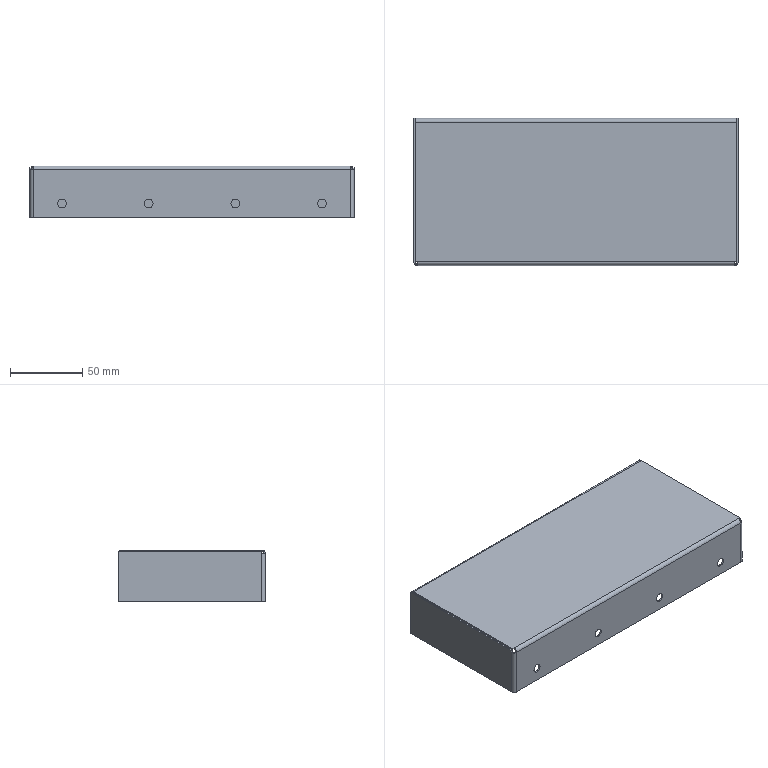Part | NX | 1 solid | 42 faces | box 225 x 102 x 36 mm | volume 44869 mm3 | plane 26 | cylinder 16 | commonest cylinder face diameters 6 x8 3.2 x4 5.2 x4
STEP:
#1=CARTESIAN_POINT('',(1610.571,113.5,87.9));
#2=VERTEX_POINT('',#1);
#3=CARTESIAN_POINT('',(1610.571,113.5,54.5));
#4=VERTEX_POINT('',#3);
#5=CARTESIAN_POINT('',(1610.571,113.5,44.938));
#6=DIRECTION('',(0.,0.,-1.));
#7=VECTOR('',#6,1000.);
#8=LINE('',#5,#7);
#9=EDGE_CURVE('',#2,#4,#8,.T.);
#10=ORIENTED_EDGE('',*,*,#9,.T.);
#11=CARTESIAN_POINT('',(1610.571,112.5,54.5));
#12=VERTEX_POINT('',#11);
#13=CARTESIAN_POINT('',(1610.571,11.5,54.5));
#14=DIRECTION('',(0.,-1.,0.));
#15=VECTOR('',#14,1000.);
#16=LINE('',#13,#15);
#17=EDGE_CURVE('',#4,#12,#16,.T.);
#18=ORIENTED_EDGE('',*,*,#17,.T.);
#19=CARTESIAN_POINT('',(1610.571,112.5,87.9));
#20=VERTEX_POINT('',#19);
#21=CARTESIAN_POINT('',(1610.571,112.5,44.938));
#22=DIRECTION('',(0.,0.,1.));
#23=VECTOR('',#22,1000.);
#24=LINE('',#21,#23);
#25=EDGE_CURVE('',#12,#20,#24,.T.);
#26=ORIENTED_EDGE('',*,*,#25,.T.);
#27=CARTESIAN_POINT('',(1610.571,110.9,89.5));
#28=VERTEX_POINT('',#27);
#29=CARTESIAN_POINT('',(1610.571,110.9,87.9));
#30=DIRECTION('',(1.,0.,0.));
#31=DIRECTION('',(0.,1.,0.));
#32=AXIS2_PLACEMENT_3D('',#29,#30,#31);
#33=CIRCLE('',#32,1.6);
#34=EDGE_CURVE('',#20,#28,#33,.T.);
#35=ORIENTED_EDGE('',*,*,#34,.T.);
#36=CARTESIAN_POINT('',(1610.571,14.1,89.5));
#37=VERTEX_POINT('',#36);
#38=CARTESIAN_POINT('',(1610.571,11.5,89.5));
#39=DIRECTION('',(0.,-1.,0.));
#40=VECTOR('',#39,1000.);
#41=LINE('',#38,#40);
#42=EDGE_CURVE('',#28,#37,#41,.T.);
#43=ORIENTED_EDGE('',*,*,#42,.T.);
#44=CARTESIAN_POINT('',(1610.571,14.1,90.5));
#45=VERTEX_POINT('',#44);
#46=CARTESIAN_POINT('',(1610.571,14.1,90.5));
#47=DIRECTION('',(0.,0.,1.));
#48=VECTOR('',#47,1000.);
#49=LINE('',#46,#48);
#50=EDGE_CURVE('',#37,#45,#49,.T.);
#51=ORIENTED_EDGE('',*,*,#50,.T.);
#52=CARTESIAN_POINT('',(1610.571,110.9,90.5));
#53=VERTEX_POINT('',#52);
#54=CARTESIAN_POINT('',(1610.571,113.5,90.5));
#55=DIRECTION('',(0.,1.,0.));
#56=VECTOR('',#55,1000.);
#57=LINE('',#54,#56);
#58=EDGE_CURVE('',#45,#53,#57,.T.);
#59=ORIENTED_EDGE('',*,*,#58,.T.);
#60=CARTESIAN_POINT('',(1610.571,110.9,87.9));
#61=DIRECTION('',(-1.,0.,0.));
#62=DIRECTION('',(0.,0.,1.));
#63=AXIS2_PLACEMENT_3D('',#60,#61,#62);
#64=CIRCLE('',#63,2.6);
#65=EDGE_CURVE('',#53,#2,#64,.T.);
#66=ORIENTED_EDGE('',*,*,#65,.T.);
#67=EDGE_LOOP('',(#10,#18,#26,#35,#43,#51,#59,#66));
#68=FACE_BOUND('',#67,.T.);
#69=CARTESIAN_POINT('',(1610.571,112.5,138.1));
#70=DIRECTION('',(-1.,0.,0.));
#71=DIRECTION('',(0.,0.,1.));
#72=AXIS2_PLACEMENT_3D('',#69,#70,#71);
#73=PLANE('',#72);
#74=ADVANCED_FACE('',(#68),#73,.T.);
#75=CARTESIAN_POINT('',(1833.5,14.1,54.5));
#76=VERTEX_POINT('',#75);
#77=CARTESIAN_POINT('',(1831.9,12.5,54.5));
#78=VERTEX_POINT('',#77);
#79=CARTESIAN_POINT('',(1831.9,14.1,54.5));
#80=DIRECTION('',(0.,0.,-1.));
#81=DIRECTION('',(1.,0.,0.));
#82=AXIS2_PLACEMENT_3D('',#79,#80,#81);
#83=CIRCLE('',#82,1.6);
#84=EDGE_CURVE('',#76,#78,#83,.T.);
#85=ORIENTED_EDGE('',*,*,#84,.F.);
#86=CARTESIAN_POINT('',(1833.5,113.5,54.5));
#87=VERTEX_POINT('',#86);
#88=CARTESIAN_POINT('',(1833.5,113.5,54.5));
#89=DIRECTION('',(0.,-1.,0.));
#90=VECTOR('',#89,1000.);
#91=LINE('',#88,#90);
#92=EDGE_CURVE('',#87,#76,#91,.T.);
#93=ORIENTED_EDGE('',*,*,#92,.F.);
#94=CARTESIAN_POINT('',(1834.5,113.5,54.5));
#95=VERTEX_POINT('',#94);
#96=CARTESIAN_POINT('',(1834.5,113.5,54.5));
#97=DIRECTION('',(-1.,0.,0.));
#98=VECTOR('',#97,1000.);
#99=LINE('',#96,#98);
#100=EDGE_CURVE('',#95,#87,#99,.T.);
#101=ORIENTED_EDGE('',*,*,#100,.F.);
#102=CARTESIAN_POINT('',(1834.5,14.1,54.5));
#103=VERTEX_POINT('',#102);
#104=CARTESIAN_POINT('',(1834.5,113.5,54.5));
#105=DIRECTION('',(0.,-1.,0.));
#106=VECTOR('',#105,1000.);
#107=LINE('',#104,#106);
#108=EDGE_CURVE('',#95,#103,#107,.T.);
#109=ORIENTED_EDGE('',*,*,#108,.T.);
#110=CARTESIAN_POINT('',(1831.9,11.5,54.5));
#111=VERTEX_POINT('',#110);
#112=CARTESIAN_POINT('',(1831.9,14.1,54.5));
#113=DIRECTION('',(0.,0.,-1.));
#114=DIRECTION('',(1.,0.,0.));
#115=AXIS2_PLACEMENT_3D('',#112,#113,#114);
#116=CIRCLE('',#115,2.6);
#117=EDGE_CURVE('',#103,#111,#116,.T.);
#118=ORIENTED_EDGE('',*,*,#117,.T.);
#119=CARTESIAN_POINT('',(1612.1,11.5,54.5));
#120=VERTEX_POINT('',#119);
#121=CARTESIAN_POINT('',(1934.4,11.5,54.5));
#122=DIRECTION('',(-1.,0.,0.));
#123=VECTOR('',#122,1000.);
#124=LINE('',#121,#123);
#125=EDGE_CURVE('',#111,#120,#124,.T.);
#126=ORIENTED_EDGE('',*,*,#125,.T.);
#127=CARTESIAN_POINT('',(1609.5,14.1,54.5));
#128=VERTEX_POINT('',#127);
#129=CARTESIAN_POINT('',(1612.1,14.1,54.5));
#130=DIRECTION('',(0.,0.,1.));
#131=DIRECTION('',(-1.,0.,0.));
#132=AXIS2_PLACEMENT_3D('',#129,#130,#131);
#133=CIRCLE('',#132,2.6);
#134=EDGE_CURVE('',#128,#120,#133,.T.);
#135=ORIENTED_EDGE('',*,*,#134,.F.);
#136=CARTESIAN_POINT('',(1609.5,113.5,54.5));
#137=VERTEX_POINT('',#136);
#138=CARTESIAN_POINT('',(1609.5,-104.365,54.5));
#139=DIRECTION('',(0.,-1.,0.));
#140=VECTOR('',#139,1000.);
#141=LINE('',#138,#140);
#142=EDGE_CURVE('',#137,#128,#141,.T.);
#143=ORIENTED_EDGE('',*,*,#142,.F.);
#144=CARTESIAN_POINT('',(1610.5,113.5,54.5));
#145=VERTEX_POINT('',#144);
#146=CARTESIAN_POINT('',(1609.5,113.5,54.5));
#147=DIRECTION('',(1.,0.,0.));
#148=VECTOR('',#147,1000.);
#149=LINE('',#146,#148);
#150=EDGE_CURVE('',#137,#145,#149,.T.);
#151=ORIENTED_EDGE('',*,*,#150,.T.);
#152=CARTESIAN_POINT('',(1610.5,14.1,54.5));
#153=VERTEX_POINT('',#152);
#154=CARTESIAN_POINT('',(1610.5,-104.365,54.5));
#155=DIRECTION('',(0.,-1.,0.));
#156=VECTOR('',#155,1000.);
#157=LINE('',#154,#156);
#158=EDGE_CURVE('',#145,#153,#157,.T.);
#159=ORIENTED_EDGE('',*,*,#158,.T.);
#160=CARTESIAN_POINT('',(1612.1,12.5,54.5));
#161=VERTEX_POINT('',#160);
#162=CARTESIAN_POINT('',(1612.1,14.1,54.5));
#163=DIRECTION('',(0.,0.,1.));
#164=DIRECTION('',(-1.,0.,0.));
#165=AXIS2_PLACEMENT_3D('',#162,#163,#164);
#166=CIRCLE('',#165,1.6);
#167=EDGE_CURVE('',#153,#161,#166,.T.);
#168=ORIENTED_EDGE('',*,*,#167,.T.);
#169=CARTESIAN_POINT('',(1934.4,12.5,54.5));
#170=DIRECTION('',(-1.,0.,0.));
#171=VECTOR('',#170,1000.);
#172=LINE('',#169,#171);
#173=EDGE_CURVE('',#78,#161,#172,.T.);
#174=ORIENTED_EDGE('',*,*,#173,.F.);
#175=EDGE_LOOP('',(#85,#93,#101,#109,#118,#126,#135,#143,#151,#159,#168,#174));
#176=FACE_BOUND('',#175,.T.);
#177=CARTESIAN_POINT('',(1831.9,14.1,54.5));
#178=DIRECTION('',(0.,0.,-1.));
#179=DIRECTION('',(0.,-1.,0.));
#180=AXIS2_PLACEMENT_3D('',#177,#178,#179);
#181=PLANE('',#180);
#182=ADVANCED_FACE('',(#176),#181,.T.);
#183=CARTESIAN_POINT('',(1833.429,112.5,54.5));
#184=VERTEX_POINT('',#183);
#185=CARTESIAN_POINT('',(1833.429,112.5,87.9));
#186=VERTEX_POINT('',#185);
#187=CARTESIAN_POINT('',(1833.429,112.5,44.938));
#188=DIRECTION('',(0.,0.,1.));
#189=VECTOR('',#188,1000.);
#190=LINE('',#187,#189);
#191=EDGE_CURVE('',#184,#186,#190,.T.);
#192=ORIENTED_EDGE('',*,*,#191,.F.);
#193=CARTESIAN_POINT('',(1833.429,113.5,54.5));
#194=VERTEX_POINT('',#193);
#195=CARTESIAN_POINT('',(1833.429,11.5,54.5));
#196=DIRECTION('',(0.,1.,0.));
#197=VECTOR('',#196,1000.);
#198=LINE('',#195,#197);
#199=EDGE_CURVE('',#184,#194,#198,.T.);
#200=ORIENTED_EDGE('',*,*,#199,.T.);
#201=CARTESIAN_POINT('',(1833.429,113.5,87.9));
#202=VERTEX_POINT('',#201);
#203=CARTESIAN_POINT('',(1833.429,113.5,44.938));
#204=DIRECTION('',(0.,0.,-1.));
#205=VECTOR('',#204,1000.);
#206=LINE('',#203,#205);
#207=EDGE_CURVE('',#202,#194,#206,.T.);
#208=ORIENTED_EDGE('',*,*,#207,.F.);
#209=CARTESIAN_POINT('',(1833.429,110.9,90.5));
#210=VERTEX_POINT('',#209);
#211=CARTESIAN_POINT('',(1833.429,110.9,87.9));
#212=DIRECTION('',(-1.,0.,0.));
#213=DIRECTION('',(0.,0.,1.));
#214=AXIS2_PLACEMENT_3D('',#211,#212,#213);
#215=CIRCLE('',#214,2.6);
#216=EDGE_CURVE('',#210,#202,#215,.T.);
#217=ORIENTED_EDGE('',*,*,#216,.F.);
#218=CARTESIAN_POINT('',(1833.429,14.1,90.5));
#219=VERTEX_POINT('',#218);
#220=CARTESIAN_POINT('',(1833.429,11.5,90.5));
#221=DIRECTION('',(0.,1.,0.));
#222=VECTOR('',#221,1000.);
#223=LINE('',#220,#222);
#224=EDGE_CURVE('',#219,#210,#223,.T.);
#225=ORIENTED_EDGE('',*,*,#224,.F.);
#226=CARTESIAN_POINT('',(1833.429,14.1,89.5));
#227=VERTEX_POINT('',#226);
#228=CARTESIAN_POINT('',(1833.429,14.1,90.5));
#229=DIRECTION('',(0.,0.,-1.));
#230=VECTOR('',#229,1000.);
#231=LINE('',#228,#230);
#232=EDGE_CURVE('',#219,#227,#231,.T.);
#233=ORIENTED_EDGE('',*,*,#232,.T.);
#234=CARTESIAN_POINT('',(1833.429,110.9,89.5));
#235=VERTEX_POINT('',#234);
#236=CARTESIAN_POINT('',(1833.429,146.329,89.5));
#237=DIRECTION('',(0.,-1.,0.));
#238=VECTOR('',#237,1000.);
#239=LINE('',#236,#238);
#240=EDGE_CURVE('',#235,#227,#239,.T.);
#241=ORIENTED_EDGE('',*,*,#240,.F.);
#242=CARTESIAN_POINT('',(1833.429,110.9,87.9));
#243=DIRECTION('',(1.,0.,0.));
#244=DIRECTION('',(0.,1.,0.));
#245=AXIS2_PLACEMENT_3D('',#242,#243,#244);
#246=CIRCLE('',#245,1.6);
#247=EDGE_CURVE('',#186,#235,#246,.T.);
#248=ORIENTED_EDGE('',*,*,#247,.F.);
#249=EDGE_LOOP('',(#192,#200,#208,#217,#225,#233,#241,#248));
#250=FACE_BOUND('',#249,.T.);
#251=CARTESIAN_POINT('',(1833.429,112.5,138.1));
#252=DIRECTION('',(1.,0.,0.));
#253=DIRECTION('',(0.,1.,0.));
#254=AXIS2_PLACEMENT_3D('',#251,#252,#253);
#255=PLANE('',#254);
#256=ADVANCED_FACE('',(#250),#255,.T.);
#257=CARTESIAN_POINT('',(1612.1,14.1,90.5));
#258=VERTEX_POINT('',#257);
#259=CARTESIAN_POINT('',(1727.465,14.1,90.5));
#260=DIRECTION('',(1.,0.,0.));
#261=VECTOR('',#260,1000.);
#262=LINE('',#259,#261);
#263=EDGE_CURVE('',#45,#258,#262,.T.);
#264=ORIENTED_EDGE('',*,*,#263,.F.);
#265=ORIENTED_EDGE('',*,*,#50,.F.);
#266=CARTESIAN_POINT('',(1612.1,14.1,89.5));
#267=VERTEX_POINT('',#266);
#268=CARTESIAN_POINT('',(1727.465,14.1,89.5));
#269=DIRECTION('',(-1.,0.,0.));
#270=VECTOR('',#269,1000.);
#271=LINE('',#268,#270);
#272=EDGE_CURVE('',#267,#37,#271,.T.);
#273=ORIENTED_EDGE('',*,*,#272,.F.);
#274=CARTESIAN_POINT('',(1612.1,14.1,90.5));
#275=DIRECTION('',(0.,0.,-1.));
#276=VECTOR('',#275,1000.);
#277=LINE('',#274,#276);
#278=EDGE_CURVE('',#258,#267,#277,.T.);
#279=ORIENTED_EDGE('',*,*,#278,.F.);
#280=EDGE_LOOP('',(#264,#265,#273,#279));
#281=FACE_BOUND('',#280,.T.);
#282=CARTESIAN_POINT('',(1609.,14.1,90.5));
#283=DIRECTION('',(0.,-1.,0.));
#284=DIRECTION('',(0.,0.,-1.));
#285=AXIS2_PLACEMENT_3D('',#282,#283,#284);
#286=PLANE('',#285);
#287=ADVANCED_FACE('',(#281),#286,.T.);
#288=CARTESIAN_POINT('',(1612.1,11.5,87.9));
#289=VERTEX_POINT('',#288);
#290=CARTESIAN_POINT('',(1609.5,14.1,87.9));
#291=VERTEX_POINT('',#290);
#292=CARTESIAN_POINT('',(1612.1,14.1,87.9));
#293=DIRECTION('',(0.,0.,-1.));
#294=DIRECTION('',(0.,-1.,0.));
#295=AXIS2_PLACEMENT_3D('',#292,#293,#294);
#296=CIRCLE('',#295,2.6);
#297=EDGE_CURVE('',#289,#291,#296,.T.);
#298=ORIENTED_EDGE('',*,*,#297,.F.);
#299=CARTESIAN_POINT('',(1612.1,12.5,87.9));
#300=VERTEX_POINT('',#299);
#301=CARTESIAN_POINT('',(1612.1,11.5,87.9));
#302=DIRECTION('',(0.,1.,0.));
#303=VECTOR('',#302,1000.);
#304=LINE('',#301,#303);
#305=EDGE_CURVE('',#289,#300,#304,.T.);
#306=ORIENTED_EDGE('',*,*,#305,.T.);
#307=CARTESIAN_POINT('',(1610.5,14.1,87.9));
#308=VERTEX_POINT('',#307);
#309=CARTESIAN_POINT('',(1612.1,14.1,87.9));
#310=DIRECTION('',(0.,0.,-1.));
#311=DIRECTION('',(0.,-1.,0.));
#312=AXIS2_PLACEMENT_3D('',#309,#310,#311);
#313=CIRCLE('',#312,1.6);
#314=EDGE_CURVE('',#300,#308,#313,.T.);
#315=ORIENTED_EDGE('',*,*,#314,.T.);
#316=CARTESIAN_POINT('',(1609.5,14.1,87.9));
#317=DIRECTION('',(1.,0.,0.));
#318=VECTOR('',#317,1000.);
#319=LINE('',#316,#318);
#320=EDGE_CURVE('',#291,#308,#319,.T.);
#321=ORIENTED_EDGE('',*,*,#320,.F.);
#322=EDGE_LOOP('',(#298,#306,#315,#321));
#323=FACE_BOUND('',#322,.T.);
#324=CARTESIAN_POINT('',(1612.1,14.1,87.9));
#325=DIRECTION('',(0.,0.,-1.));
#326=DIRECTION('',(0.,-1.,0.));
#327=AXIS2_PLACEMENT_3D('',#324,#325,#326);
#328=PLANE('',#327);
#329=ADVANCED_FACE('',(#323),#328,.F.);
#330=CARTESIAN_POINT('',(1635.,11.5,64.5));
#331=VERTEX_POINT('',#330);
#332=CARTESIAN_POINT('',(1629.,11.5,64.5));
#333=VERTEX_POINT('',#332);
#334=CARTESIAN_POINT('',(1632.,11.5,64.5));
#335=DIRECTION('',(0.,1.,0.));
#336=DIRECTION('',(1.,0.,0.));
#337=AXIS2_PLACEMENT_3D('',#334,#335,#336);
#338=CIRCLE('',#337,3.);
#339=EDGE_CURVE('',#331,#333,#338,.T.);
#340=ORIENTED_EDGE('',*,*,#339,.F.);
#341=CARTESIAN_POINT('',(1635.,12.5,64.5));
#342=VERTEX_POINT('',#341);
#343=CARTESIAN_POINT('',(1635.,12.6,64.5));
#344=DIRECTION('',(0.,1.,0.));
#345=VECTOR('',#344,1000.);
#346=LINE('',#343,#345);
#347=EDGE_CURVE('',#331,#342,#346,.T.);
#348=ORIENTED_EDGE('',*,*,#347,.T.);
#349=CARTESIAN_POINT('',(1629.,12.5,64.5));
#350=VERTEX_POINT('',#349);
#351=CARTESIAN_POINT('',(1632.,12.5,64.5));
#352=DIRECTION('',(0.,1.,0.));
#353=DIRECTION('',(1.,0.,0.));
#354=AXIS2_PLACEMENT_3D('',#351,#352,#353);
#355=CIRCLE('',#354,3.);
#356=EDGE_CURVE('',#342,#350,#355,.T.);
#357=ORIENTED_EDGE('',*,*,#356,.T.);
#358=CARTESIAN_POINT('',(1629.,12.6,64.5));
#359=DIRECTION('',(0.,1.,0.));
#360=VECTOR('',#359,1000.);
#361=LINE('',#358,#360);
#362=EDGE_CURVE('',#333,#350,#361,.T.);
#363=ORIENTED_EDGE('',*,*,#362,.F.);
#364=EDGE_LOOP('',(#340,#348,#357,#363));
#365=FACE_BOUND('',#364,.T.);
#366=CARTESIAN_POINT('',(1632.,12.6,64.5));
#367=DIRECTION('',(0.,1.,0.));
#368=DIRECTION('',(1.,0.,0.));
#369=AXIS2_PLACEMENT_3D('',#366,#367,#368);
#370=CYLINDRICAL_SURFACE('',#369,3.);
#371=ADVANCED_FACE('',(#365),#370,.F.);
#372=CARTESIAN_POINT('',(1809.,11.5,64.5));
#373=VERTEX_POINT('',#372);
#374=CARTESIAN_POINT('',(1815.,11.5,64.5));
#375=VERTEX_POINT('',#374);
#376=CARTESIAN_POINT('',(1812.,11.5,64.5));
#377=DIRECTION('',(0.,1.,0.));
#378=DIRECTION('',(1.,0.,0.));
#379=AXIS2_PLACEMENT_3D('',#376,#377,#378);
#380=CIRCLE('',#379,3.);
#381=EDGE_CURVE('',#373,#375,#380,.T.);
#382=ORIENTED_EDGE('',*,*,#381,.F.);
#383=CARTESIAN_POINT('',(1809.,12.5,64.5));
#384=VERTEX_POINT('',#383);
#385=CARTESIAN_POINT('',(1809.,12.6,64.5));
#386=DIRECTION('',(0.,1.,0.));
#387=VECTOR('',#386,1000.);
#388=LINE('',#385,#387);
#389=EDGE_CURVE('',#384,#373,#388,.F.);
#390=ORIENTED_EDGE('',*,*,#389,.F.);
#391=CARTESIAN_POINT('',(1815.,12.5,64.5));
#392=VERTEX_POINT('',#391);
#393=CARTESIAN_POINT('',(1812.,12.5,64.5));
#394=DIRECTION('',(0.,1.,0.));
#395=DIRECTION('',(1.,0.,0.));
#396=AXIS2_PLACEMENT_3D('',#393,#394,#395);
#397=CIRCLE('',#396,3.);
#398=EDGE_CURVE('',#384,#392,#397,.T.);
#399=ORIENTED_EDGE('',*,*,#398,.T.);
#400=CARTESIAN_POINT('',(1815.,12.6,64.5));
#401=DIRECTION('',(0.,1.,0.));
#402=VECTOR('',#401,1000.);
#403=LINE('',#400,#402);
#404=EDGE_CURVE('',#392,#375,#403,.F.);
#405=ORIENTED_EDGE('',*,*,#404,.T.);
#406=EDGE_LOOP('',(#382,#390,#399,#405));
#407=FACE_BOUND('',#406,.T.);
#408=CARTESIAN_POINT('',(1812.,12.6,64.5));
#409=DIRECTION('',(0.,1.,0.));
#410=DIRECTION('',(1.,0.,0.));
#411=AXIS2_PLACEMENT_3D('',#408,#409,#410);
#412=CYLINDRICAL_SURFACE('',#411,3.);
#413=ADVANCED_FACE('',(#407),#412,.F.);
#414=CARTESIAN_POINT('',(1695.,11.5,64.5));
#415=VERTEX_POINT('',#414);
#416=CARTESIAN_POINT('',(1689.,11.5,64.5));
#417=VERTEX_POINT('',#416);
#418=CARTESIAN_POINT('',(1692.,11.5,64.5));
#419=DIRECTION('',(0.,1.,0.));
#420=DIRECTION('',(1.,0.,0.));
#421=AXIS2_PLACEMENT_3D('',#418,#419,#420);
#422=CIRCLE('',#421,3.);
#423=EDGE_CURVE('',#415,#417,#422,.T.);
#424=ORIENTED_EDGE('',*,*,#423,.F.);
#425=CARTESIAN_POINT('',(1695.,12.5,64.5));
#426=VERTEX_POINT('',#425);
#427=CARTESIAN_POINT('',(1695.,12.6,64.5));
#428=DIRECTION('',(0.,1.,0.));
#429=VECTOR('',#428,1000.);
#430=LINE('',#427,#429);
#431=EDGE_CURVE('',#415,#426,#430,.T.);
#432=ORIENTED_EDGE('',*,*,#431,.T.);
#433=CARTESIAN_POINT('',(1689.,12.5,64.5));
#434=VERTEX_POINT('',#433);
#435=CARTESIAN_POINT('',(1692.,12.5,64.5));
#436=DIRECTION('',(0.,1.,0.));
#437=DIRECTION('',(1.,0.,0.));
#438=AXIS2_PLACEMENT_3D('',#435,#436,#437);
#439=CIRCLE('',#438,3.);
#440=EDGE_CURVE('',#426,#434,#439,.T.);
#441=ORIENTED_EDGE('',*,*,#440,.T.);
#442=CARTESIAN_POINT('',(1689.,12.6,64.5));
#443=DIRECTION('',(0.,1.,0.));
#444=VECTOR('',#443,1000.);
#445=LINE('',#442,#444);
#446=EDGE_CURVE('',#417,#434,#445,.T.);
#447=ORIENTED_EDGE('',*,*,#446,.F.);
#448=EDGE_LOOP('',(#424,#432,#441,#447));
#449=FACE_BOUND('',#448,.T.);
#450=CARTESIAN_POINT('',(1692.,12.6,64.5));
#451=DIRECTION('',(0.,1.,0.));
#452=DIRECTION('',(1.,0.,0.));
#453=AXIS2_PLACEMENT_3D('',#450,#451,#452);
#454=CYLINDRICAL_SURFACE('',#453,3.);
#455=ADVANCED_FACE('',(#449),#454,.F.);
#456=CARTESIAN_POINT('',(1749.,12.5,64.5));
#457=VERTEX_POINT('',#456);
#458=CARTESIAN_POINT('',(1755.,12.5,64.5));
#459=VERTEX_POINT('',#458);
#460=CARTESIAN_POINT('',(1752.,12.5,64.5));
#461=DIRECTION('',(0.,1.,0.));
#462=DIRECTION('',(1.,0.,0.));
#463=AXIS2_PLACEMENT_3D('',#460,#461,#462);
#464=CIRCLE('',#463,3.);
#465=EDGE_CURVE('',#457,#459,#464,.T.);
#466=ORIENTED_EDGE('',*,*,#465,.T.);
#467=CARTESIAN_POINT('',(1755.,11.5,64.5));
#468=VERTEX_POINT('',#467);
#469=CARTESIAN_POINT('',(1755.,12.6,64.5));
#470=DIRECTION('',(0.,1.,0.));
#471=VECTOR('',#470,1000.);
#472=LINE('',#469,#471);
#473=EDGE_CURVE('',#468,#459,#472,.T.);
#474=ORIENTED_EDGE('',*,*,#473,.F.);
#475=CARTESIAN_POINT('',(1749.,11.5,64.5));
#476=VERTEX_POINT('',#475);
#477=CARTESIAN_POINT('',(1752.,11.5,64.5));
#478=DIRECTION('',(0.,1.,0.));
#479=DIRECTION('',(1.,0.,0.));
#480=AXIS2_PLACEMENT_3D('',#477,#478,#479);
#481=CIRCLE('',#480,3.);
#482=EDGE_CURVE('',#476,#468,#481,.T.);
#483=ORIENTED_EDGE('',*,*,#482,.F.);
#484=CARTESIAN_POINT('',(1749.,12.6,64.5));
#485=DIRECTION('',(0.,1.,0.));
#486=VECTOR('',#485,1000.);
#487=LINE('',#484,#486);
#488=EDGE_CURVE('',#476,#457,#487,.T.);
#489=ORIENTED_EDGE('',*,*,#488,.T.);
#490=EDGE_LOOP('',(#466,#474,#483,#489));
#491=FACE_BOUND('',#490,.T.);
#492=CARTESIAN_POINT('',(1752.,12.6,64.5));
#493=DIRECTION('',(0.,1.,0.));
#494=DIRECTION('',(1.,0.,0.));
#495=AXIS2_PLACEMENT_3D('',#492,#493,#494);
#496=CYLINDRICAL_SURFACE('',#495,3.);
#497=ADVANCED_FACE('',(#491),#496,.F.);
#498=CARTESIAN_POINT('',(1834.5,14.1,87.9));
#499=VERTEX_POINT('',#498);
#500=CARTESIAN_POINT('',(1831.9,11.5,87.9));
#501=VERTEX_POINT('',#500);
#502=CARTESIAN_POINT('',(1831.9,14.1,87.9));
#503=DIRECTION('',(0.,0.,-1.));
#504=DIRECTION('',(1.,0.,0.));
#505=AXIS2_PLACEMENT_3D('',#502,#503,#504);
#506=CIRCLE('',#505,2.6);
#507=EDGE_CURVE('',#499,#501,#506,.T.);
#508=ORIENTED_EDGE('',*,*,#507,.F.);
#509=CARTESIAN_POINT('',(1833.5,14.1,87.9));
#510=VERTEX_POINT('',#509);
#511=CARTESIAN_POINT('',(1834.5,14.1,87.9));
#512=DIRECTION('',(-1.,0.,0.));
#513=VECTOR('',#512,1000.);
#514=LINE('',#511,#513);
#515=EDGE_CURVE('',#499,#510,#514,.T.);
#516=ORIENTED_EDGE('',*,*,#515,.T.);
#517=CARTESIAN_POINT('',(1831.9,12.5,87.9));
#518=VERTEX_POINT('',#517);
#519=CARTESIAN_POINT('',(1831.9,14.1,87.9));
#520=DIRECTION('',(0.,0.,-1.));
#521=DIRECTION('',(1.,0.,0.));
#522=AXIS2_PLACEMENT_3D('',#519,#520,#521);
#523=CIRCLE('',#522,1.6);
#524=EDGE_CURVE('',#510,#518,#523,.T.);
#525=ORIENTED_EDGE('',*,*,#524,.T.);
#526=CARTESIAN_POINT('',(1831.9,11.5,87.9));
#527=DIRECTION('',(0.,1.,0.));
#528=VECTOR('',#527,1000.);
#529=LINE('',#526,#528);
#530=EDGE_CURVE('',#501,#518,#529,.T.);
#531=ORIENTED_EDGE('',*,*,#530,.F.);
#532=EDGE_LOOP('',(#508,#516,#525,#531));
#533=FACE_BOUND('',#532,.T.);
#534=CARTESIAN_POINT('',(1831.9,14.1,87.9));
#535=DIRECTION('',(0.,0.,-1.));
#536=DIRECTION('',(0.,-1.,0.));
#537=AXIS2_PLACEMENT_3D('',#534,#535,#536);
#538=PLANE('',#537);
#539=ADVANCED_FACE('',(#533),#538,.F.);
#540=CARTESIAN_POINT('',(1831.9,14.1,90.5));
#541=VERTEX_POINT('',#540);
#542=CARTESIAN_POINT('',(1831.9,14.1,87.9));
#543=DIRECTION('',(-1.,0.,0.));
#544=DIRECTION('',(0.,-1.,0.));
#545=AXIS2_PLACEMENT_3D('',#542,#543,#544);
#546=CIRCLE('',#545,2.6);
#547=EDGE_CURVE('',#501,#541,#546,.T.);
#548=ORIENTED_EDGE('',*,*,#547,.F.);
#549=ORIENTED_EDGE('',*,*,#530,.T.);
#550=CARTESIAN_POINT('',(1831.9,14.1,89.5));
#551=VERTEX_POINT('',#550);
#552=CARTESIAN_POINT('',(1831.9,14.1,87.9));
#553=DIRECTION('',(1.,0.,0.));
#554=DIRECTION('',(0.,0.,1.));
#555=AXIS2_PLACEMENT_3D('',#552,#553,#554);
#556=CIRCLE('',#555,1.6);
#557=EDGE_CURVE('',#551,#518,#556,.T.);
#558=ORIENTED_EDGE('',*,*,#557,.F.);
#559=CARTESIAN_POINT('',(1831.9,14.1,90.5));
#560=DIRECTION('',(0.,0.,-1.));
#561=VECTOR('',#560,1000.);
#562=LINE('',#559,#561);
#563=EDGE_CURVE('',#541,#551,#562,.T.);
#564=ORIENTED_EDGE('',*,*,#563,.F.);
#565=EDGE_LOOP('',(#548,#549,#558,#564));
#566=FACE_BOUND('',#565,.T.);
#567=CARTESIAN_POINT('',(1831.9,14.1,87.9));
#568=DIRECTION('',(-1.,0.,0.));
#569=DIRECTION('',(0.,0.,1.));
#570=AXIS2_PLACEMENT_3D('',#567,#568,#569);
#571=PLANE('',#570);
#572=ADVANCED_FACE('',(#566),#571,.F.);
#573=ORIENTED_EDGE('',*,*,#547,.T.);
#574=CARTESIAN_POINT('',(1831.9,14.1,90.5));
#575=DIRECTION('',(1.,0.,0.));
#576=VECTOR('',#575,1000.);
#577=LINE('',#574,#576);
#578=EDGE_CURVE('',#258,#541,#577,.T.);
#579=ORIENTED_EDGE('',*,*,#578,.F.);
#580=CARTESIAN_POINT('',(1612.1,14.1,87.9));
#581=DIRECTION('',(1.,0.,0.));
#582=DIRECTION('',(0.,0.,1.));
#583=AXIS2_PLACEMENT_3D('',#580,#581,#582);
#584=CIRCLE('',#583,2.6);
#585=EDGE_CURVE('',#258,#289,#584,.T.);
#586=ORIENTED_EDGE('',*,*,#585,.T.);
#587=CARTESIAN_POINT('',(1727.465,11.5,87.9));
#588=DIRECTION('',(1.,0.,0.));
#589=VECTOR('',#588,1000.);
#590=LINE('',#587,#589);
#591=EDGE_CURVE('',#289,#501,#590,.T.);
#592=ORIENTED_EDGE('',*,*,#591,.T.);
#593=EDGE_LOOP('',(#573,#579,#586,#592));
#594=FACE_BOUND('',#593,.T.);
#595=CARTESIAN_POINT('',(1831.9,14.1,87.9));
#596=DIRECTION('',(1.,0.,0.));
#597=DIRECTION('',(0.,0.,-1.));
#598=AXIS2_PLACEMENT_3D('',#595,#596,#597);
#599=CYLINDRICAL_SURFACE('',#598,2.6);
#600=ADVANCED_FACE('',(#594),#599,.T.);
#601=ORIENTED_EDGE('',*,*,#207,.T.);
#602=CARTESIAN_POINT('',(1727.465,113.5,54.5));
#603=DIRECTION('',(-1.,0.,0.));
#604=VECTOR('',#603,1000.);
#605=LINE('',#602,#604);
#606=EDGE_CURVE('',#194,#4,#605,.T.);
#607=ORIENTED_EDGE('',*,*,#606,.T.);
#608=ORIENTED_EDGE('',*,*,#9,.F.);
#609=CARTESIAN_POINT('',(1727.465,113.5,87.9));
#610=DIRECTION('',(1.,0.,0.));
#611=VECTOR('',#610,1000.);
#612=LINE('',#609,#611);
#613=EDGE_CURVE('',#2,#202,#612,.T.);
#614=ORIENTED_EDGE('',*,*,#613,.T.);
#615=EDGE_LOOP('',(#601,#607,#608,#614));
#616=FACE_BOUND('',#615,.T.);
#617=CARTESIAN_POINT('',(1727.465,113.5,233.862));
#618=DIRECTION('',(0.,1.,0.));
#619=DIRECTION('',(1.,0.,0.));
#620=AXIS2_PLACEMENT_3D('',#617,#618,#619);
#621=PLANE('',#620);
#622=ADVANCED_FACE('',(#616),#621,.T.);
#623=CARTESIAN_POINT('',(1833.429,110.9,90.5));
#624=DIRECTION('',(1.,0.,0.));
#625=VECTOR('',#624,1000.);
#626=LINE('',#623,#625);
#627=EDGE_CURVE('',#53,#210,#626,.T.);
#628=ORIENTED_EDGE('',*,*,#627,.F.);
#629=ORIENTED_EDGE('',*,*,#58,.F.);
#630=ORIENTED_EDGE('',*,*,#263,.T.);
#631=ORIENTED_EDGE('',*,*,#578,.T.);
#632=CARTESIAN_POINT('',(1727.465,14.1,90.5));
#633=DIRECTION('',(1.,0.,0.));
#634=VECTOR('',#633,1000.);
#635=LINE('',#632,#634);
#636=EDGE_CURVE('',#541,#219,#635,.T.);
#637=ORIENTED_EDGE('',*,*,#636,.T.);
#638=ORIENTED_EDGE('',*,*,#224,.T.);
#639=EDGE_LOOP('',(#628,#629,#630,#631,#637,#638));
#640=FACE_BOUND('',#639,.T.);
#641=CARTESIAN_POINT('',(1727.465,-31.962,90.5));
#642=DIRECTION('',(0.,0.,1.));
#643=DIRECTION('',(1.,0.,0.));
#644=AXIS2_PLACEMENT_3D('',#641,#642,#643);
#645=PLANE('',#644);
#646=ADVANCED_FACE('',(#640),#645,.T.);
#647=ORIENTED_EDGE('',*,*,#613,.F.);
#648=ORIENTED_EDGE('',*,*,#65,.F.);
#649=ORIENTED_EDGE('',*,*,#627,.T.);
#650=ORIENTED_EDGE('',*,*,#216,.T.);
#651=EDGE_LOOP('',(#647,#648,#649,#650));
#652=FACE_BOUND('',#651,.T.);
#653=CARTESIAN_POINT('',(1833.429,110.9,87.9));
#654=DIRECTION('',(1.,0.,0.));
#655=DIRECTION('',(0.,0.,-1.));
#656=AXIS2_PLACEMENT_3D('',#653,#654,#655);
#657=CYLINDRICAL_SURFACE('',#656,2.6);
#658=ADVANCED_FACE('',(#652),#657,.T.);
#659=CARTESIAN_POINT('',(1610.5,14.1,87.9));
#660=DIRECTION('',(0.,0.,1.));
#661=VECTOR('',#660,1000.);
#662=LINE('',#659,#661);
#663=EDGE_CURVE('',#153,#308,#662,.T.);
#664=ORIENTED_EDGE('',*,*,#663,.F.);
#665=ORIENTED_EDGE('',*,*,#158,.F.);
#666=CARTESIAN_POINT('',(1610.5,113.5,89.429));
#667=VERTEX_POINT('',#666);
#668=CARTESIAN_POINT('',(1610.5,113.5,54.5));
#669=DIRECTION('',(0.,0.,1.));
#670=VECTOR('',#669,1000.);
#671=LINE('',#668,#670);
#672=EDGE_CURVE('',#145,#667,#671,.T.);
#673=ORIENTED_EDGE('',*,*,#672,.T.);
#674=CARTESIAN_POINT('',(1610.5,14.1,89.429));
#675=VERTEX_POINT('',#674);
#676=CARTESIAN_POINT('',(1610.5,113.5,89.429));
#677=DIRECTION('',(0.,-1.,0.));
#678=VECTOR('',#677,1000.);
#679=LINE('',#676,#678);
#680=EDGE_CURVE('',#667,#675,#679,.T.);
#681=ORIENTED_EDGE('',*,*,#680,.T.);
#682=CARTESIAN_POINT('',(1610.5,14.1,44.938));
#683=DIRECTION('',(0.,0.,1.));
#684=VECTOR('',#683,1000.);
#685=LINE('',#682,#684);
#686=EDGE_CURVE('',#308,#675,#685,.T.);
#687=ORIENTED_EDGE('',*,*,#686,.F.);
#688=EDGE_LOOP('',(#664,#665,#673,#681,#687));
#689=FACE_BOUND('',#688,.T.);
#690=CARTESIAN_POINT('',(1610.5,13.1,90.5));
#691=DIRECTION('',(-1.,0.,0.));
#692=DIRECTION('',(0.,0.,1.));
#693=AXIS2_PLACEMENT_3D('',#690,#691,#692);
#694=PLANE('',#693);
#695=ADVANCED_FACE('',(#689),#694,.F.);
#696=ORIENTED_EDGE('',*,*,#314,.F.);
#697=CARTESIAN_POINT('',(1612.1,12.5,44.938));
#698=DIRECTION('',(0.,0.,1.));
#699=VECTOR('',#698,1000.);
#700=LINE('',#697,#699);
#701=EDGE_CURVE('',#161,#300,#700,.T.);
#702=ORIENTED_EDGE('',*,*,#701,.F.);
#703=ORIENTED_EDGE('',*,*,#167,.F.);
#704=ORIENTED_EDGE('',*,*,#663,.T.);
#705=EDGE_LOOP('',(#696,#702,#703,#704));
#706=FACE_BOUND('',#705,.T.);
#707=CARTESIAN_POINT('',(1612.1,14.1,87.9));
#708=DIRECTION('',(0.,0.,1.));
#709=DIRECTION('',(1.,0.,0.));
#710=AXIS2_PLACEMENT_3D('',#707,#708,#709);
#711=CYLINDRICAL_SURFACE('',#710,1.6);
#712=ADVANCED_FACE('',(#706),#711,.F.);
#713=ORIENTED_EDGE('',*,*,#557,.T.);
#714=CARTESIAN_POINT('',(1727.465,12.5,87.9));
#715=DIRECTION('',(1.,0.,0.));
#716=VECTOR('',#715,1000.);
#717=LINE('',#714,#716);
#718=EDGE_CURVE('',#300,#518,#717,.T.);
#719=ORIENTED_EDGE('',*,*,#718,.F.);
#720=CARTESIAN_POINT('',(1612.1,14.1,87.9));
#721=DIRECTION('',(-1.,0.,0.));
#722=DIRECTION('',(0.,-1.,0.));
#723=AXIS2_PLACEMENT_3D('',#720,#721,#722);
#724=CIRCLE('',#723,1.6);
#725=EDGE_CURVE('',#300,#267,#724,.T.);
#726=ORIENTED_EDGE('',*,*,#725,.T.);
#727=CARTESIAN_POINT('',(1831.9,14.1,89.5));
#728=DIRECTION('',(1.,0.,0.));
#729=VECTOR('',#728,1000.);
#730=LINE('',#727,#729);
#731=EDGE_CURVE('',#267,#551,#730,.T.);
#732=ORIENTED_EDGE('',*,*,#731,.T.);
#733=EDGE_LOOP('',(#713,#719,#726,#732));
#734=FACE_BOUND('',#733,.T.);
#735=CARTESIAN_POINT('',(1831.9,14.1,87.9));
#736=DIRECTION('',(1.,0.,0.));
#737=DIRECTION('',(0.,0.,-1.));
#738=AXIS2_PLACEMENT_3D('',#735,#736,#737);
#739=CYLINDRICAL_SURFACE('',#738,1.6);
#740=ADVANCED_FACE('',(#734),#739,.F.);
#741=ORIENTED_EDGE('',*,*,#636,.F.);
#742=ORIENTED_EDGE('',*,*,#563,.T.);
#743=CARTESIAN_POINT('',(1727.465,14.1,89.5));
#744=DIRECTION('',(-1.,0.,0.));
#745=VECTOR('',#744,1000.);
#746=LINE('',#743,#745);
#747=EDGE_CURVE('',#227,#551,#746,.T.);
#748=ORIENTED_EDGE('',*,*,#747,.F.);
#749=ORIENTED_EDGE('',*,*,#232,.F.);
#750=EDGE_LOOP('',(#741,#742,#748,#749));
#751=FACE_BOUND('',#750,.T.);
#752=CARTESIAN_POINT('',(1831.9,14.1,90.5));
#753=DIRECTION('',(0.,-1.,0.));
#754=DIRECTION('',(0.,0.,-1.));
#755=AXIS2_PLACEMENT_3D('',#752,#753,#754);
#756=PLANE('',#755);
#757=ADVANCED_FACE('',(#751),#756,.T.);
#758=CARTESIAN_POINT('',(1609.5,113.5,89.429));
#759=VERTEX_POINT('',#758);
#760=CARTESIAN_POINT('',(1609.5,113.5,54.5));
#761=DIRECTION('',(0.,0.,1.));
#762=VECTOR('',#761,1000.);
#763=LINE('',#760,#762);
#764=EDGE_CURVE('',#137,#759,#763,.T.);
#765=ORIENTED_EDGE('',*,*,#764,.T.);
#766=CARTESIAN_POINT('',(1609.5,113.5,89.429));
#767=DIRECTION('',(1.,0.,0.));
#768=VECTOR('',#767,1000.);
#769=LINE('',#766,#768);
#770=EDGE_CURVE('',#759,#667,#769,.T.);
#771=ORIENTED_EDGE('',*,*,#770,.T.);
#772=ORIENTED_EDGE('',*,*,#672,.F.);
#773=ORIENTED_EDGE('',*,*,#150,.F.);
#774=EDGE_LOOP('',(#765,#771,#772,#773));
#775=FACE_BOUND('',#774,.T.);
#776=CARTESIAN_POINT('',(1609.5,113.5,89.429));
#777=DIRECTION('',(0.,1.,0.));
#778=DIRECTION('',(1.,0.,0.));
#779=AXIS2_PLACEMENT_3D('',#776,#777,#778);
#780=PLANE('',#779);
#781=ADVANCED_FACE('',(#775),#780,.T.);
#782=CARTESIAN_POINT('',(1609.5,14.1,89.429));
#783=VERTEX_POINT('',#782);
#784=CARTESIAN_POINT('',(1609.5,14.1,89.429));
#785=DIRECTION('',(1.,0.,0.));
#786=VECTOR('',#785,1000.);
#787=LINE('',#784,#786);
#788=EDGE_CURVE('',#783,#675,#787,.T.);
#789=ORIENTED_EDGE('',*,*,#788,.T.);
#790=ORIENTED_EDGE('',*,*,#680,.F.);
#791=ORIENTED_EDGE('',*,*,#770,.F.);
#792=CARTESIAN_POINT('',(1609.5,113.5,89.429));
#793=DIRECTION('',(0.,-1.,0.));
#794=VECTOR('',#793,1000.);
#795=LINE('',#792,#794);
#796=EDGE_CURVE('',#759,#783,#795,.T.);
#797=ORIENTED_EDGE('',*,*,#796,.T.);
#798=EDGE_LOOP('',(#789,#790,#791,#797));
#799=FACE_BOUND('',#798,.T.);
#800=CARTESIAN_POINT('',(1609.5,13.6,89.429));
#801=DIRECTION('',(0.,0.,1.));
#802=DIRECTION('',(0.,-1.,0.));
#803=AXIS2_PLACEMENT_3D('',#800,#801,#802);
#804=PLANE('',#803);
#805=ADVANCED_FACE('',(#799),#804,.T.);
#806=ORIENTED_EDGE('',*,*,#788,.F.);
#807=CARTESIAN_POINT('',(1609.5,14.1,44.938));
#808=DIRECTION('',(0.,0.,1.));
#809=VECTOR('',#808,1000.);
#810=LINE('',#807,#809);
#811=EDGE_CURVE('',#291,#783,#810,.T.);
#812=ORIENTED_EDGE('',*,*,#811,.F.);
#813=ORIENTED_EDGE('',*,*,#320,.T.);
#814=ORIENTED_EDGE('',*,*,#686,.T.);
#815=EDGE_LOOP('',(#806,#812,#813,#814));
#816=FACE_BOUND('',#815,.T.);
#817=CARTESIAN_POINT('',(1609.5,14.1,87.9));
#818=DIRECTION('',(0.,-1.,0.));
#819=DIRECTION('',(0.,0.,-1.));
#820=AXIS2_PLACEMENT_3D('',#817,#818,#819);
#821=PLANE('',#820);
#822=ADVANCED_FACE('',(#816),#821,.T.);
#823=ORIENTED_EDGE('',*,*,#297,.T.);
#824=CARTESIAN_POINT('',(1609.5,14.1,87.9));
#825=DIRECTION('',(0.,0.,1.));
#826=VECTOR('',#825,1000.);
#827=LINE('',#824,#826);
#828=EDGE_CURVE('',#128,#291,#827,.T.);
#829=ORIENTED_EDGE('',*,*,#828,.F.);
#830=ORIENTED_EDGE('',*,*,#134,.T.);
#831=CARTESIAN_POINT('',(1612.1,11.5,44.938));
#832=DIRECTION('',(0.,0.,1.));
#833=VECTOR('',#832,1000.);
#834=LINE('',#831,#833);
#835=EDGE_CURVE('',#120,#289,#834,.T.);
#836=ORIENTED_EDGE('',*,*,#835,.T.);
#837=EDGE_LOOP('',(#823,#829,#830,#836));
#838=FACE_BOUND('',#837,.T.);
#839=CARTESIAN_POINT('',(1612.1,14.1,87.9));
#840=DIRECTION('',(0.,0.,1.));
#841=DIRECTION('',(1.,0.,0.));
#842=AXIS2_PLACEMENT_3D('',#839,#840,#841);
#843=CYLINDRICAL_SURFACE('',#842,2.6);
#844=ADVANCED_FACE('',(#838),#843,.T.);
#845=ORIENTED_EDGE('',*,*,#835,.F.);
#846=ORIENTED_EDGE('',*,*,#125,.F.);
#847=CARTESIAN_POINT('',(1831.9,11.5,44.938));
#848=DIRECTION('',(0.,0.,-1.));
#849=VECTOR('',#848,1000.);
#850=LINE('',#847,#849);
#851=EDGE_CURVE('',#501,#111,#850,.T.);
#852=ORIENTED_EDGE('',*,*,#851,.F.);
#853=ORIENTED_EDGE('',*,*,#591,.F.);
#854=EDGE_LOOP('',(#845,#846,#852,#853));
#855=FACE_BOUND('',#854,.T.);
#856=ORIENTED_EDGE('',*,*,#423,.T.);
#857=CARTESIAN_POINT('',(1692.,11.5,64.5));
#858=DIRECTION('',(0.,1.,0.));
#859=DIRECTION('',(1.,0.,0.));
#860=AXIS2_PLACEMENT_3D('',#857,#858,#859);
#861=CIRCLE('',#860,3.);
#862=EDGE_CURVE('',#417,#415,#861,.T.);
#863=ORIENTED_EDGE('',*,*,#862,.T.);
#864=EDGE_LOOP('',(#856,#863));
#865=FACE_BOUND('',#864,.T.);
#866=ORIENTED_EDGE('',*,*,#339,.T.);
#867=CARTESIAN_POINT('',(1632.,11.5,64.5));
#868=DIRECTION('',(0.,1.,0.));
#869=DIRECTION('',(1.,0.,0.));
#870=AXIS2_PLACEMENT_3D('',#867,#868,#869);
#871=CIRCLE('',#870,3.);
#872=EDGE_CURVE('',#333,#331,#871,.T.);
#873=ORIENTED_EDGE('',*,*,#872,.T.);
#874=EDGE_LOOP('',(#866,#873));
#875=FACE_BOUND('',#874,.T.);
#876=ORIENTED_EDGE('',*,*,#482,.T.);
#877=CARTESIAN_POINT('',(1752.,11.5,64.5));
#878=DIRECTION('',(0.,1.,0.));
#879=DIRECTION('',(1.,0.,0.));
#880=AXIS2_PLACEMENT_3D('',#877,#878,#879);
#881=CIRCLE('',#880,3.);
#882=EDGE_CURVE('',#468,#476,#881,.T.);
#883=ORIENTED_EDGE('',*,*,#882,.T.);
#884=EDGE_LOOP('',(#876,#883));
#885=FACE_BOUND('',#884,.T.);
#886=ORIENTED_EDGE('',*,*,#381,.T.);
#887=CARTESIAN_POINT('',(1812.,11.5,64.5));
#888=DIRECTION('',(0.,1.,0.));
#889=DIRECTION('',(1.,0.,0.));
#890=AXIS2_PLACEMENT_3D('',#887,#888,#889);
#891=CIRCLE('',#890,3.);
#892=EDGE_CURVE('',#375,#373,#891,.T.);
#893=ORIENTED_EDGE('',*,*,#892,.T.);
#894=EDGE_LOOP('',(#886,#893));
#895=FACE_BOUND('',#894,.T.);
#896=CARTESIAN_POINT('',(1609.5,11.5,54.5));
#897=DIRECTION('',(0.,-1.,0.));
#898=DIRECTION('',(0.,0.,-1.));
#899=AXIS2_PLACEMENT_3D('',#896,#897,#898);
#900=PLANE('',#899);
#901=ADVANCED_FACE('',(#855,#865,#875,#885,#895),#900,.T.);
#902=ORIENTED_EDGE('',*,*,#828,.T.);
#903=ORIENTED_EDGE('',*,*,#811,.T.);
#904=ORIENTED_EDGE('',*,*,#796,.F.);
#905=ORIENTED_EDGE('',*,*,#764,.F.);
#906=ORIENTED_EDGE('',*,*,#142,.T.);
#907=EDGE_LOOP('',(#902,#903,#904,#905,#906));
#908=FACE_BOUND('',#907,.T.);
#909=CARTESIAN_POINT('',(1609.5,13.6,54.5));
#910=DIRECTION('',(-1.,0.,0.));
#911=DIRECTION('',(0.,0.,1.));
#912=AXIS2_PLACEMENT_3D('',#909,#910,#911);
#913=PLANE('',#912);
#914=ADVANCED_FACE('',(#908),#913,.T.);
#915=ORIENTED_EDGE('',*,*,#851,.T.);
#916=ORIENTED_EDGE('',*,*,#117,.F.);
#917=CARTESIAN_POINT('',(1834.5,14.1,54.5));
#918=DIRECTION('',(0.,0.,-1.));
#919=VECTOR('',#918,1000.);
#920=LINE('',#917,#919);
#921=EDGE_CURVE('',#499,#103,#920,.T.);
#922=ORIENTED_EDGE('',*,*,#921,.F.);
#923=ORIENTED_EDGE('',*,*,#507,.T.);
#924=EDGE_LOOP('',(#915,#916,#922,#923));
#925=FACE_BOUND('',#924,.T.);
#926=CARTESIAN_POINT('',(1831.9,14.1,54.5));
#927=DIRECTION('',(0.,0.,-1.));
#928=DIRECTION('',(-1.,0.,0.));
#929=AXIS2_PLACEMENT_3D('',#926,#927,#928);
#930=CYLINDRICAL_SURFACE('',#929,2.6);
#931=ADVANCED_FACE('',(#925),#930,.T.);
#932=ORIENTED_EDGE('',*,*,#921,.T.);
#933=ORIENTED_EDGE('',*,*,#108,.F.);
#934=CARTESIAN_POINT('',(1834.5,113.5,89.429));
#935=VERTEX_POINT('',#934);
#936=CARTESIAN_POINT('',(1834.5,113.5,89.429));
#937=DIRECTION('',(0.,0.,-1.));
#938=VECTOR('',#937,1000.);
#939=LINE('',#936,#938);
#940=EDGE_CURVE('',#935,#95,#939,.T.);
#941=ORIENTED_EDGE('',*,*,#940,.F.);
#942=CARTESIAN_POINT('',(1834.5,14.1,89.429));
#943=VERTEX_POINT('',#942);
#944=CARTESIAN_POINT('',(1834.5,13.6,89.429));
#945=DIRECTION('',(0.,1.,0.));
#946=VECTOR('',#945,1000.);
#947=LINE('',#944,#946);
#948=EDGE_CURVE('',#943,#935,#947,.T.);
#949=ORIENTED_EDGE('',*,*,#948,.F.);
#950=CARTESIAN_POINT('',(1834.5,14.1,44.938));
#951=DIRECTION('',(0.,0.,-1.));
#952=VECTOR('',#951,1000.);
#953=LINE('',#950,#952);
#954=EDGE_CURVE('',#943,#499,#953,.T.);
#955=ORIENTED_EDGE('',*,*,#954,.T.);
#956=EDGE_LOOP('',(#932,#933,#941,#949,#955));
#957=FACE_BOUND('',#956,.T.);
#958=CARTESIAN_POINT('',(1834.5,-211.4,54.5));
#959=DIRECTION('',(1.,0.,0.));
#960=DIRECTION('',(0.,1.,0.));
#961=AXIS2_PLACEMENT_3D('',#958,#959,#960);
#962=PLANE('',#961);
#963=ADVANCED_FACE('',(#957),#962,.T.);
#964=CARTESIAN_POINT('',(1833.5,14.1,89.429));
#965=VERTEX_POINT('',#964);
#966=CARTESIAN_POINT('',(1834.5,14.1,89.429));
#967=DIRECTION('',(1.,0.,0.));
#968=VECTOR('',#967,1000.);
#969=LINE('',#966,#968);
#970=EDGE_CURVE('',#965,#943,#969,.T.);
#971=ORIENTED_EDGE('',*,*,#970,.F.);
#972=CARTESIAN_POINT('',(1833.5,14.1,44.938));
#973=DIRECTION('',(0.,0.,-1.));
#974=VECTOR('',#973,1000.);
#975=LINE('',#972,#974);
#976=EDGE_CURVE('',#965,#510,#975,.T.);
#977=ORIENTED_EDGE('',*,*,#976,.T.);
#978=ORIENTED_EDGE('',*,*,#515,.F.);
#979=ORIENTED_EDGE('',*,*,#954,.F.);
#980=EDGE_LOOP('',(#971,#977,#978,#979));
#981=FACE_BOUND('',#980,.T.);
#982=CARTESIAN_POINT('',(1834.5,14.1,91.));
#983=DIRECTION('',(0.,-1.,0.));
#984=DIRECTION('',(0.,0.,-1.));
#985=AXIS2_PLACEMENT_3D('',#982,#983,#984);
#986=PLANE('',#985);
#987=ADVANCED_FACE('',(#981),#986,.T.);
#988=CARTESIAN_POINT('',(1833.5,113.5,89.429));
#989=VERTEX_POINT('',#988);
#990=CARTESIAN_POINT('',(1833.5,13.6,89.429));
#991=DIRECTION('',(0.,1.,0.));
#992=VECTOR('',#991,1000.);
#993=LINE('',#990,#992);
#994=EDGE_CURVE('',#965,#989,#993,.T.);
#995=ORIENTED_EDGE('',*,*,#994,.T.);
#996=CARTESIAN_POINT('',(1833.5,113.5,89.429));
#997=DIRECTION('',(0.,0.,-1.));
#998=VECTOR('',#997,1000.);
#999=LINE('',#996,#998);
#1000=EDGE_CURVE('',#989,#87,#999,.T.);
#1001=ORIENTED_EDGE('',*,*,#1000,.T.);
#1002=ORIENTED_EDGE('',*,*,#92,.T.);
#1003=CARTESIAN_POINT('',(1833.5,14.1,54.5));
#1004=DIRECTION('',(0.,0.,-1.));
#1005=VECTOR('',#1004,1000.);
#1006=LINE('',#1003,#1005);
#1007=EDGE_CURVE('',#510,#76,#1006,.T.);
#1008=ORIENTED_EDGE('',*,*,#1007,.F.);
#1009=ORIENTED_EDGE('',*,*,#976,.F.);
#1010=EDGE_LOOP('',(#995,#1001,#1002,#1008,#1009));
#1011=FACE_BOUND('',#1010,.T.);
#1012=CARTESIAN_POINT('',(1833.5,13.6,87.9));
#1013=DIRECTION('',(1.,0.,0.));
#1014=DIRECTION('',(0.,1.,0.));
#1015=AXIS2_PLACEMENT_3D('',#1012,#1013,#1014);
#1016=PLANE('',#1015);
#1017=ADVANCED_FACE('',(#1011),#1016,.F.);
#1018=ORIENTED_EDGE('',*,*,#948,.T.);
#1019=CARTESIAN_POINT('',(1834.5,113.5,89.429));
#1020=DIRECTION('',(-1.,0.,0.));
#1021=VECTOR('',#1020,1000.);
#1022=LINE('',#1019,#1021);
#1023=EDGE_CURVE('',#935,#989,#1022,.T.);
#1024=ORIENTED_EDGE('',*,*,#1023,.T.);
#1025=ORIENTED_EDGE('',*,*,#994,.F.);
#1026=ORIENTED_EDGE('',*,*,#970,.T.);
#1027=EDGE_LOOP('',(#1018,#1024,#1025,#1026));
#1028=FACE_BOUND('',#1027,.T.);
#1029=CARTESIAN_POINT('',(1834.5,113.5,89.429));
#1030=DIRECTION('',(0.,0.,1.));
#1031=DIRECTION('',(0.,-1.,0.));
#1032=AXIS2_PLACEMENT_3D('',#1029,#1030,#1031);
#1033=PLANE('',#1032);
#1034=ADVANCED_FACE('',(#1028),#1033,.T.);
#1035=ORIENTED_EDGE('',*,*,#940,.T.);
#1036=ORIENTED_EDGE('',*,*,#100,.T.);
#1037=ORIENTED_EDGE('',*,*,#1000,.F.);
#1038=ORIENTED_EDGE('',*,*,#1023,.F.);
#1039=EDGE_LOOP('',(#1035,#1036,#1037,#1038));
#1040=FACE_BOUND('',#1039,.T.);
#1041=CARTESIAN_POINT('',(1834.5,113.5,54.5));
#1042=DIRECTION('',(0.,1.,0.));
#1043=DIRECTION('',(1.,0.,0.));
#1044=AXIS2_PLACEMENT_3D('',#1041,#1042,#1043);
#1045=PLANE('',#1044);
#1046=ADVANCED_FACE('',(#1040),#1045,.T.);
#1047=CARTESIAN_POINT('',(1831.9,12.5,44.938));
#1048=DIRECTION('',(0.,0.,-1.));
#1049=VECTOR('',#1048,1000.);
#1050=LINE('',#1047,#1049);
#1051=EDGE_CURVE('',#518,#78,#1050,.T.);
#1052=ORIENTED_EDGE('',*,*,#1051,.T.);
#1053=ORIENTED_EDGE('',*,*,#173,.T.);
#1054=ORIENTED_EDGE('',*,*,#701,.T.);
#1055=ORIENTED_EDGE('',*,*,#718,.T.);
#1056=EDGE_LOOP('',(#1052,#1053,#1054,#1055));
#1057=FACE_BOUND('',#1056,.T.);
#1058=CARTESIAN_POINT('',(1692.,12.5,64.5));
#1059=DIRECTION('',(0.,1.,0.));
#1060=DIRECTION('',(1.,0.,0.));
#1061=AXIS2_PLACEMENT_3D('',#1058,#1059,#1060);
#1062=CIRCLE('',#1061,3.);
#1063=EDGE_CURVE('',#434,#426,#1062,.T.);
#1064=ORIENTED_EDGE('',*,*,#1063,.F.);
#1065=ORIENTED_EDGE('',*,*,#440,.F.);
#1066=EDGE_LOOP('',(#1064,#1065));
#1067=FACE_BOUND('',#1066,.T.);
#1068=CARTESIAN_POINT('',(1812.,12.5,64.5));
#1069=DIRECTION('',(0.,1.,0.));
#1070=DIRECTION('',(1.,0.,0.));
#1071=AXIS2_PLACEMENT_3D('',#1068,#1069,#1070);
#1072=CIRCLE('',#1071,3.);
#1073=EDGE_CURVE('',#392,#384,#1072,.T.);
#1074=ORIENTED_EDGE('',*,*,#1073,.F.);
#1075=ORIENTED_EDGE('',*,*,#398,.F.);
#1076=EDGE_LOOP('',(#1074,#1075));
#1077=FACE_BOUND('',#1076,.T.);
#1078=CARTESIAN_POINT('',(1632.,12.5,64.5));
#1079=DIRECTION('',(0.,1.,0.));
#1080=DIRECTION('',(1.,0.,0.));
#1081=AXIS2_PLACEMENT_3D('',#1078,#1079,#1080);
#1082=CIRCLE('',#1081,3.);
#1083=EDGE_CURVE('',#350,#342,#1082,.T.);
#1084=ORIENTED_EDGE('',*,*,#1083,.F.);
#1085=ORIENTED_EDGE('',*,*,#356,.F.);
#1086=EDGE_LOOP('',(#1084,#1085));
#1087=FACE_BOUND('',#1086,.T.);
#1088=ORIENTED_EDGE('',*,*,#465,.F.);
#1089=CARTESIAN_POINT('',(1752.,12.5,64.5));
#1090=DIRECTION('',(0.,1.,0.));
#1091=DIRECTION('',(1.,0.,0.));
#1092=AXIS2_PLACEMENT_3D('',#1089,#1090,#1091);
#1093=CIRCLE('',#1092,3.);
#1094=EDGE_CURVE('',#459,#457,#1093,.T.);
#1095=ORIENTED_EDGE('',*,*,#1094,.F.);
#1096=EDGE_LOOP('',(#1088,#1095));
#1097=FACE_BOUND('',#1096,.T.);
#1098=CARTESIAN_POINT('',(1834.5,12.5,87.9));
#1099=DIRECTION('',(0.,-1.,0.));
#1100=DIRECTION('',(0.,0.,-1.));
#1101=AXIS2_PLACEMENT_3D('',#1098,#1099,#1100);
#1102=PLANE('',#1101);
#1103=ADVANCED_FACE('',(#1057,#1067,#1077,#1087,#1097),#1102,.F.);
#1104=ORIENTED_EDGE('',*,*,#1007,.T.);
#1105=ORIENTED_EDGE('',*,*,#84,.T.);
#1106=ORIENTED_EDGE('',*,*,#1051,.F.);
#1107=ORIENTED_EDGE('',*,*,#524,.F.);
#1108=EDGE_LOOP('',(#1104,#1105,#1106,#1107));
#1109=FACE_BOUND('',#1108,.T.);
#1110=CARTESIAN_POINT('',(1831.9,14.1,54.5));
#1111=DIRECTION('',(0.,0.,-1.));
#1112=DIRECTION('',(-1.,0.,0.));
#1113=AXIS2_PLACEMENT_3D('',#1110,#1111,#1112);
#1114=CYLINDRICAL_SURFACE('',#1113,1.6);
#1115=ADVANCED_FACE('',(#1109),#1114,.F.);
#1116=ORIENTED_EDGE('',*,*,#606,.F.);
#1117=ORIENTED_EDGE('',*,*,#199,.F.);
#1118=CARTESIAN_POINT('',(1727.465,112.5,54.5));
#1119=DIRECTION('',(-1.,0.,0.));
#1120=VECTOR('',#1119,1000.);
#1121=LINE('',#1118,#1120);
#1122=EDGE_CURVE('',#184,#12,#1121,.T.);
#1123=ORIENTED_EDGE('',*,*,#1122,.T.);
#1124=ORIENTED_EDGE('',*,*,#17,.F.);
#1125=EDGE_LOOP('',(#1116,#1117,#1123,#1124));
#1126=FACE_BOUND('',#1125,.T.);
#1127=CARTESIAN_POINT('',(1833.429,113.5,54.5));
#1128=DIRECTION('',(0.,0.,-1.));
#1129=DIRECTION('',(0.,-1.,0.));
#1130=AXIS2_PLACEMENT_3D('',#1127,#1128,#1129);
#1131=PLANE('',#1130);
#1132=ADVANCED_FACE('',(#1126),#1131,.T.);
#1133=ORIENTED_EDGE('',*,*,#42,.F.);
#1134=CARTESIAN_POINT('',(1833.429,110.9,89.5));
#1135=DIRECTION('',(1.,0.,0.));
#1136=VECTOR('',#1135,1000.);
#1137=LINE('',#1134,#1136);
#1138=EDGE_CURVE('',#28,#235,#1137,.T.);
#1139=ORIENTED_EDGE('',*,*,#1138,.T.);
#1140=ORIENTED_EDGE('',*,*,#240,.T.);
#1141=ORIENTED_EDGE('',*,*,#747,.T.);
#1142=ORIENTED_EDGE('',*,*,#731,.F.);
#1143=ORIENTED_EDGE('',*,*,#272,.T.);
#1144=EDGE_LOOP('',(#1133,#1139,#1140,#1141,#1142,#1143));
#1145=FACE_BOUND('',#1144,.T.);
#1146=CARTESIAN_POINT('',(1610.571,113.5,89.5));
#1147=DIRECTION('',(0.,0.,1.));
#1148=DIRECTION('',(1.,0.,0.));
#1149=AXIS2_PLACEMENT_3D('',#1146,#1147,#1148);
#1150=PLANE('',#1149);
#1151=ADVANCED_FACE('',(#1145),#1150,.F.);
#1152=ORIENTED_EDGE('',*,*,#1138,.F.);
#1153=ORIENTED_EDGE('',*,*,#34,.F.);
#1154=CARTESIAN_POINT('',(1727.465,112.5,87.9));
#1155=DIRECTION('',(1.,0.,0.));
#1156=VECTOR('',#1155,1000.);
#1157=LINE('',#1154,#1156);
#1158=EDGE_CURVE('',#20,#186,#1157,.T.);
#1159=ORIENTED_EDGE('',*,*,#1158,.T.);
#1160=ORIENTED_EDGE('',*,*,#247,.T.);
#1161=EDGE_LOOP('',(#1152,#1153,#1159,#1160));
#1162=FACE_BOUND('',#1161,.T.);
#1163=CARTESIAN_POINT('',(1833.429,110.9,87.9));
#1164=DIRECTION('',(1.,0.,0.));
#1165=DIRECTION('',(0.,0.,-1.));
#1166=AXIS2_PLACEMENT_3D('',#1163,#1164,#1165);
#1167=CYLINDRICAL_SURFACE('',#1166,1.6);
#1168=ADVANCED_FACE('',(#1162),#1167,.F.);
#1169=ORIENTED_EDGE('',*,*,#1158,.F.);
#1170=ORIENTED_EDGE('',*,*,#25,.F.);
#1171=ORIENTED_EDGE('',*,*,#1122,.F.);
#1172=ORIENTED_EDGE('',*,*,#191,.T.);
#1173=EDGE_LOOP('',(#1169,#1170,#1171,#1172));
#1174=FACE_BOUND('',#1173,.T.);
#1175=CARTESIAN_POINT('',(1610.571,112.5,88.4));
#1176=DIRECTION('',(0.,1.,0.));
#1177=DIRECTION('',(1.,0.,0.));
#1178=AXIS2_PLACEMENT_3D('',#1175,#1176,#1177);
#1179=PLANE('',#1178);
#1180=ADVANCED_FACE('',(#1174),#1179,.F.);
#1181=ORIENTED_EDGE('',*,*,#585,.F.);
#1182=ORIENTED_EDGE('',*,*,#278,.T.);
#1183=ORIENTED_EDGE('',*,*,#725,.F.);
#1184=ORIENTED_EDGE('',*,*,#305,.F.);
#1185=EDGE_LOOP('',(#1181,#1182,#1183,#1184));
#1186=FACE_BOUND('',#1185,.T.);
#1187=CARTESIAN_POINT('',(1612.1,14.1,87.9));
#1188=DIRECTION('',(1.,0.,0.));
#1189=DIRECTION('',(0.,1.,0.));
#1190=AXIS2_PLACEMENT_3D('',#1187,#1188,#1189);
#1191=PLANE('',#1190);
#1192=ADVANCED_FACE('',(#1186),#1191,.F.);
#1193=ORIENTED_EDGE('',*,*,#473,.T.);
#1194=ORIENTED_EDGE('',*,*,#1094,.T.);
#1195=ORIENTED_EDGE('',*,*,#488,.F.);
#1196=ORIENTED_EDGE('',*,*,#882,.F.);
#1197=EDGE_LOOP('',(#1193,#1194,#1195,#1196));
#1198=FACE_BOUND('',#1197,.T.);
#1199=CARTESIAN_POINT('',(1752.,12.6,64.5));
#1200=DIRECTION('',(0.,1.,0.));
#1201=DIRECTION('',(1.,0.,0.));
#1202=AXIS2_PLACEMENT_3D('',#1199,#1200,#1201);
#1203=CYLINDRICAL_SURFACE('',#1202,3.);
#1204=ADVANCED_FACE('',(#1198),#1203,.F.);
#1205=ORIENTED_EDGE('',*,*,#1083,.T.);
#1206=ORIENTED_EDGE('',*,*,#347,.F.);
#1207=ORIENTED_EDGE('',*,*,#872,.F.);
#1208=ORIENTED_EDGE('',*,*,#362,.T.);
#1209=EDGE_LOOP('',(#1205,#1206,#1207,#1208));
#1210=FACE_BOUND('',#1209,.T.);
#1211=CARTESIAN_POINT('',(1632.,12.6,64.5));
#1212=DIRECTION('',(0.,1.,0.));
#1213=DIRECTION('',(1.,0.,0.));
#1214=AXIS2_PLACEMENT_3D('',#1211,#1212,#1213);
#1215=CYLINDRICAL_SURFACE('',#1214,3.);
#1216=ADVANCED_FACE('',(#1210),#1215,.F.);
#1217=ORIENTED_EDGE('',*,*,#1073,.T.);
#1218=ORIENTED_EDGE('',*,*,#389,.T.);
#1219=ORIENTED_EDGE('',*,*,#892,.F.);
#1220=ORIENTED_EDGE('',*,*,#404,.F.);
#1221=EDGE_LOOP('',(#1217,#1218,#1219,#1220));
#1222=FACE_BOUND('',#1221,.T.);
#1223=CARTESIAN_POINT('',(1812.,12.6,64.5));
#1224=DIRECTION('',(0.,1.,0.));
#1225=DIRECTION('',(1.,0.,0.));
#1226=AXIS2_PLACEMENT_3D('',#1223,#1224,#1225);
#1227=CYLINDRICAL_SURFACE('',#1226,3.);
#1228=ADVANCED_FACE('',(#1222),#1227,.F.);
#1229=ORIENTED_EDGE('',*,*,#1063,.T.);
#1230=ORIENTED_EDGE('',*,*,#431,.F.);
#1231=ORIENTED_EDGE('',*,*,#862,.F.);
#1232=ORIENTED_EDGE('',*,*,#446,.T.);
#1233=EDGE_LOOP('',(#1229,#1230,#1231,#1232));
#1234=FACE_BOUND('',#1233,.T.);
#1235=CARTESIAN_POINT('',(1692.,12.6,64.5));
#1236=DIRECTION('',(0.,1.,0.));
#1237=DIRECTION('',(1.,0.,0.));
#1238=AXIS2_PLACEMENT_3D('',#1235,#1236,#1237);
#1239=CYLINDRICAL_SURFACE('',#1238,3.);
#1240=ADVANCED_FACE('',(#1234),#1239,.F.);
#1241=CLOSED_SHELL('',(#74,#182,#256,#287,#329,#371,#413,#455,#497,#539,#572,#600,#622,#646,#658,#695,#712,#740,#757,#781,#805,#822,#844,#901,#914,#931,#963,#987,#1017,#1034,#1046,#1103,#1115,#1132,#1151,#1168,#1180,#1192,#1204,#1216,#1228,#1240));
#1242=MANIFOLD_SOLID_BREP('',#1241);
#1243=(LENGTH_UNIT()NAMED_UNIT(*)SI_UNIT(.MILLI.,.METRE.));
#1244=UNCERTAINTY_MEASURE_WITH_UNIT(LENGTH_MEASURE(0.00001),#1243,'','');
#1245=(NAMED_UNIT(*)PLANE_ANGLE_UNIT()SI_UNIT($,.RADIAN.));
#1246=(NAMED_UNIT(*)SI_UNIT($,.STERADIAN.)SOLID_ANGLE_UNIT());
#1247=(GEOMETRIC_REPRESENTATION_CONTEXT(3)GLOBAL_UNCERTAINTY_ASSIGNED_CONTEXT((#1244))GLOBAL_UNIT_ASSIGNED_CONTEXT((#1243,#1245,#1246))REPRESENTATION_CONTEXT('',''));
#1248=ADVANCED_BREP_SHAPE_REPRESENTATION('',(#1242),#1247);